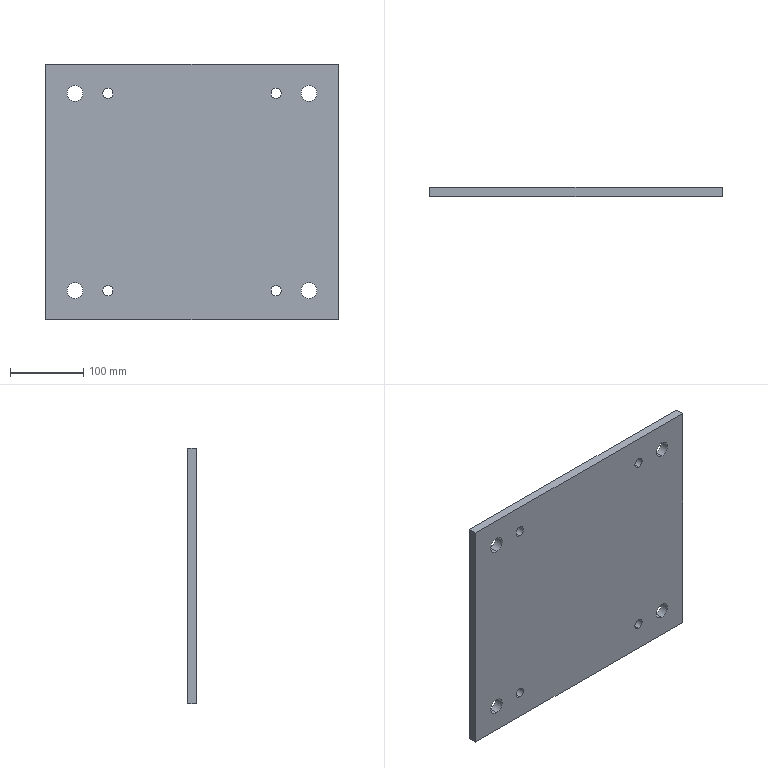Part | STEP file | 立柱底Plate-200×150 | 1 solid | 22 faces | box 400 x 12 x 350 mm | volume 1654365 mm3 | cylinder 16 | plane 6 | commonest cylinder face diameters 14 x8 22 x8